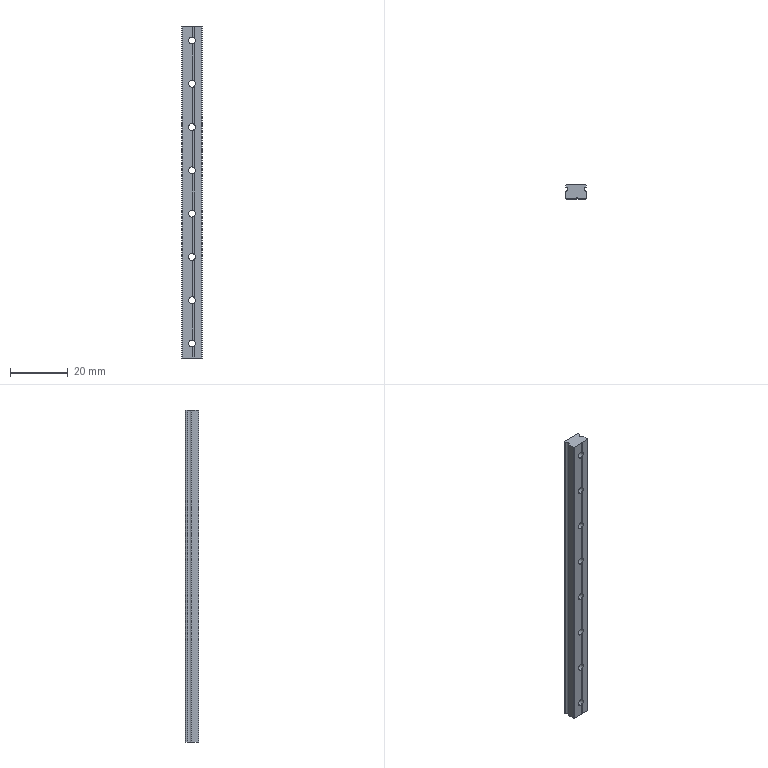Part | STEP file | MGN7C-rail L115 | 1 solid | 65 faces | box 7 x 4.8 x 115 mm | volume 3319 mm3 | cylinder 44 | plane 21 | commonest cylinder face diameters 2.4 x16 4.2 x16 0.6 x9 1.4 x3